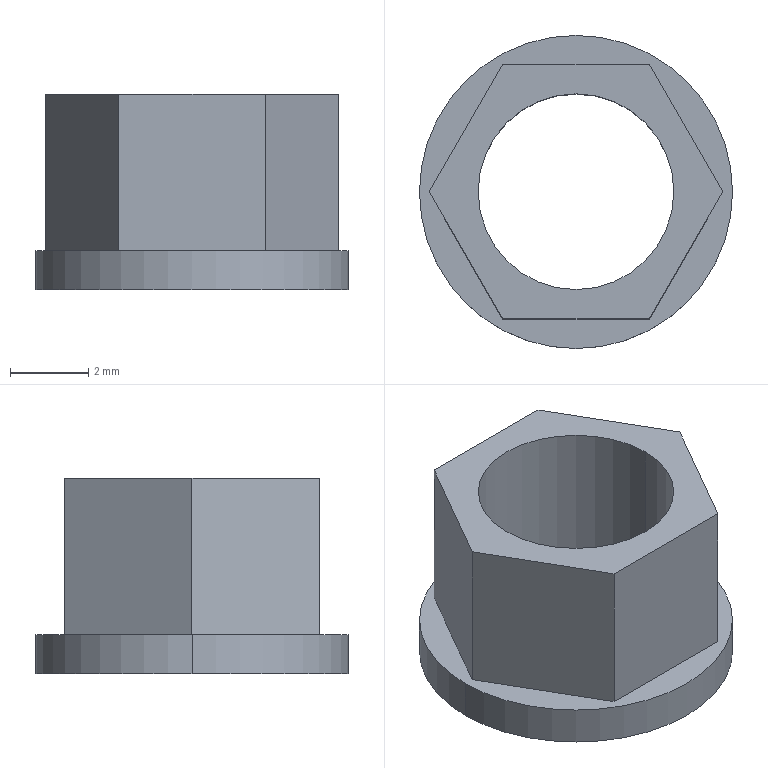Part | SolidWorks | features BaseBody 1 | 1 solid | 13 faces | box 8 x 8 x 5 mm | volume 98.449 mm3 | plane 9 | cylinder 4 | commonest cylinder face diameters 5 x2 8 x2
STEP:
#1=CARTESIAN_POINT('',(2.5,0.,0.));
#2=VERTEX_POINT('',#1);
#3=CARTESIAN_POINT('',(-2.5,0.,0.));
#4=VERTEX_POINT('',#3);
#5=CARTESIAN_POINT('',(0.,0.,0.));
#6=DIRECTION('',(0.,0.,1.));
#7=DIRECTION('',(-1.,0.,0.));
#8=AXIS2_PLACEMENT_3D('',#5,#6,#7);
#9=CIRCLE('',#8,2.5);
#10=EDGE_CURVE('',#2,#4,#9,.T.);
#11=ORIENTED_EDGE('',*,*,#10,.F.);
#12=CARTESIAN_POINT('',(2.5,0.,5.));
#13=VERTEX_POINT('',#12);
#14=CARTESIAN_POINT('',(2.5,0.,5.));
#15=DIRECTION('',(0.,0.,1.));
#16=VECTOR('',#15,1000.);
#17=LINE('',#14,#16);
#18=EDGE_CURVE('',#2,#13,#17,.T.);
#19=ORIENTED_EDGE('',*,*,#18,.T.);
#20=CARTESIAN_POINT('',(-2.5,0.,5.));
#21=VERTEX_POINT('',#20);
#22=CARTESIAN_POINT('',(0.,0.,5.));
#23=DIRECTION('',(0.,0.,-1.));
#24=DIRECTION('',(-1.,0.,0.));
#25=AXIS2_PLACEMENT_3D('',#22,#23,#24);
#26=CIRCLE('',#25,2.5);
#27=EDGE_CURVE('',#21,#13,#26,.T.);
#28=ORIENTED_EDGE('',*,*,#27,.F.);
#29=CARTESIAN_POINT('',(-2.5,0.,5.));
#30=DIRECTION('',(0.,0.,1.));
#31=VECTOR('',#30,1000.);
#32=LINE('',#29,#31);
#33=EDGE_CURVE('',#4,#21,#32,.T.);
#34=ORIENTED_EDGE('',*,*,#33,.F.);
#35=EDGE_LOOP('',(#11,#19,#28,#34));
#36=FACE_OUTER_BOUND('',#35,.T.);
#37=CARTESIAN_POINT('',(0.,0.,5.));
#38=DIRECTION('',(0.,0.,1.));
#39=DIRECTION('',(-1.,0.,0.));
#40=AXIS2_PLACEMENT_3D('',#37,#38,#39);
#41=CYLINDRICAL_SURFACE('',#40,2.5);
#42=ADVANCED_FACE('',(#36),#41,.F.);
#43=CARTESIAN_POINT('',(4.,0.,1.));
#44=VERTEX_POINT('',#43);
#45=CARTESIAN_POINT('',(-4.,0.,1.));
#46=VERTEX_POINT('',#45);
#47=CARTESIAN_POINT('',(0.,0.,1.));
#48=DIRECTION('',(0.,0.,1.));
#49=DIRECTION('',(-1.,0.,0.));
#50=AXIS2_PLACEMENT_3D('',#47,#48,#49);
#51=CIRCLE('',#50,4.);
#52=EDGE_CURVE('',#44,#46,#51,.T.);
#53=ORIENTED_EDGE('',*,*,#52,.F.);
#54=CARTESIAN_POINT('',(4.,0.,0.));
#55=VERTEX_POINT('',#54);
#56=CARTESIAN_POINT('',(4.,0.,0.));
#57=DIRECTION('',(0.,0.,-1.));
#58=VECTOR('',#57,1000.);
#59=LINE('',#56,#58);
#60=EDGE_CURVE('',#44,#55,#59,.T.);
#61=ORIENTED_EDGE('',*,*,#60,.T.);
#62=CARTESIAN_POINT('',(-4.,0.,0.));
#63=VERTEX_POINT('',#62);
#64=CARTESIAN_POINT('',(0.,0.,0.));
#65=DIRECTION('',(0.,0.,-1.));
#66=DIRECTION('',(-1.,0.,0.));
#67=AXIS2_PLACEMENT_3D('',#64,#65,#66);
#68=CIRCLE('',#67,4.);
#69=EDGE_CURVE('',#63,#55,#68,.T.);
#70=ORIENTED_EDGE('',*,*,#69,.F.);
#71=CARTESIAN_POINT('',(-4.,0.,0.));
#72=DIRECTION('',(0.,0.,-1.));
#73=VECTOR('',#72,1000.);
#74=LINE('',#71,#73);
#75=EDGE_CURVE('',#46,#63,#74,.T.);
#76=ORIENTED_EDGE('',*,*,#75,.F.);
#77=EDGE_LOOP('',(#53,#61,#70,#76));
#78=FACE_OUTER_BOUND('',#77,.T.);
#79=CARTESIAN_POINT('',(0.,0.,0.));
#80=DIRECTION('',(0.,0.,-1.));
#81=DIRECTION('',(-1.,0.,0.));
#82=AXIS2_PLACEMENT_3D('',#79,#80,#81);
#83=CYLINDRICAL_SURFACE('',#82,4.);
#84=ADVANCED_FACE('',(#78),#83,.T.);
#85=CARTESIAN_POINT('',(-1.876,-3.25,1.));
#86=VERTEX_POINT('',#85);
#87=CARTESIAN_POINT('',(-3.753,0.,1.));
#88=VERTEX_POINT('',#87);
#89=CARTESIAN_POINT('',(-3.284,-0.8125,1.));
#90=DIRECTION('',(-0.5,0.866,0.));
#91=VECTOR('',#90,1000.);
#92=LINE('',#89,#91);
#93=EDGE_CURVE('',#86,#88,#92,.T.);
#94=ORIENTED_EDGE('',*,*,#93,.F.);
#95=CARTESIAN_POINT('',(-1.876,-3.25,5.));
#96=VERTEX_POINT('',#95);
#97=CARTESIAN_POINT('',(-1.876,-3.25,1.));
#98=DIRECTION('',(0.,0.,1.));
#99=VECTOR('',#98,1000.);
#100=LINE('',#97,#99);
#101=EDGE_CURVE('',#86,#96,#100,.T.);
#102=ORIENTED_EDGE('',*,*,#101,.T.);
#103=CARTESIAN_POINT('',(-3.753,0.,5.));
#104=VERTEX_POINT('',#103);
#105=CARTESIAN_POINT('',(-1.876,-3.25,5.));
#106=DIRECTION('',(0.5,-0.866,0.));
#107=VECTOR('',#106,1000.);
#108=LINE('',#105,#107);
#109=EDGE_CURVE('',#104,#96,#108,.T.);
#110=ORIENTED_EDGE('',*,*,#109,.F.);
#111=CARTESIAN_POINT('',(-3.753,0.,1.));
#112=DIRECTION('',(0.,0.,1.));
#113=VECTOR('',#112,1000.);
#114=LINE('',#111,#113);
#115=EDGE_CURVE('',#88,#104,#114,.T.);
#116=ORIENTED_EDGE('',*,*,#115,.F.);
#117=EDGE_LOOP('',(#94,#102,#110,#116));
#118=FACE_OUTER_BOUND('',#117,.T.);
#119=CARTESIAN_POINT('',(-3.753,0.,1.));
#120=DIRECTION('',(-0.866,-0.5,0.));
#121=DIRECTION('',(-0.5,0.866,0.));
#122=AXIS2_PLACEMENT_3D('',#119,#120,#121);
#123=PLANE('',#122);
#124=ADVANCED_FACE('',(#118),#123,.T.);
#125=CARTESIAN_POINT('',(-1.876,3.25,1.));
#126=VERTEX_POINT('',#125);
#127=CARTESIAN_POINT('',(-2.345,2.438,1.));
#128=DIRECTION('',(0.5,0.866,0.));
#129=VECTOR('',#128,1000.);
#130=LINE('',#127,#129);
#131=EDGE_CURVE('',#88,#126,#130,.T.);
#132=ORIENTED_EDGE('',*,*,#131,.F.);
#133=ORIENTED_EDGE('',*,*,#115,.T.);
#134=CARTESIAN_POINT('',(-1.876,3.25,5.));
#135=VERTEX_POINT('',#134);
#136=CARTESIAN_POINT('',(-3.753,0.,5.));
#137=DIRECTION('',(-0.5,-0.866,0.));
#138=VECTOR('',#137,1000.);
#139=LINE('',#136,#138);
#140=EDGE_CURVE('',#135,#104,#139,.T.);
#141=ORIENTED_EDGE('',*,*,#140,.F.);
#142=CARTESIAN_POINT('',(-1.876,3.25,1.));
#143=DIRECTION('',(0.,0.,1.));
#144=VECTOR('',#143,1000.);
#145=LINE('',#142,#144);
#146=EDGE_CURVE('',#126,#135,#145,.T.);
#147=ORIENTED_EDGE('',*,*,#146,.F.);
#148=EDGE_LOOP('',(#132,#133,#141,#147));
#149=FACE_OUTER_BOUND('',#148,.T.);
#150=CARTESIAN_POINT('',(-1.876,3.25,1.));
#151=DIRECTION('',(-0.866,0.5,0.));
#152=DIRECTION('',(0.,0.,1.));
#153=AXIS2_PLACEMENT_3D('',#150,#151,#152);
#154=PLANE('',#153);
#155=ADVANCED_FACE('',(#149),#154,.T.);
#156=CARTESIAN_POINT('',(1.876,3.25,1.));
#157=VERTEX_POINT('',#156);
#158=CARTESIAN_POINT('',(0.9382,3.25,1.));
#159=DIRECTION('',(1.,0.,0.));
#160=VECTOR('',#159,1000.);
#161=LINE('',#158,#160);
#162=EDGE_CURVE('',#126,#157,#161,.T.);
#163=ORIENTED_EDGE('',*,*,#162,.F.);
#164=ORIENTED_EDGE('',*,*,#146,.T.);
#165=CARTESIAN_POINT('',(1.876,3.25,5.));
#166=VERTEX_POINT('',#165);
#167=CARTESIAN_POINT('',(-1.876,3.25,5.));
#168=DIRECTION('',(-1.,0.,0.));
#169=VECTOR('',#168,1000.);
#170=LINE('',#167,#169);
#171=EDGE_CURVE('',#166,#135,#170,.T.);
#172=ORIENTED_EDGE('',*,*,#171,.F.);
#173=CARTESIAN_POINT('',(1.876,3.25,1.));
#174=DIRECTION('',(0.,0.,1.));
#175=VECTOR('',#174,1000.);
#176=LINE('',#173,#175);
#177=EDGE_CURVE('',#157,#166,#176,.T.);
#178=ORIENTED_EDGE('',*,*,#177,.F.);
#179=EDGE_LOOP('',(#163,#164,#172,#178));
#180=FACE_OUTER_BOUND('',#179,.T.);
#181=CARTESIAN_POINT('',(1.876,3.25,1.));
#182=DIRECTION('',(0.,1.,0.));
#183=DIRECTION('',(1.,0.,0.));
#184=AXIS2_PLACEMENT_3D('',#181,#182,#183);
#185=PLANE('',#184);
#186=ADVANCED_FACE('',(#180),#185,.T.);
#187=CARTESIAN_POINT('',(3.753,0.,1.));
#188=VERTEX_POINT('',#187);
#189=CARTESIAN_POINT('',(3.284,0.8125,1.));
#190=DIRECTION('',(0.5,-0.866,0.));
#191=VECTOR('',#190,1000.);
#192=LINE('',#189,#191);
#193=EDGE_CURVE('',#157,#188,#192,.T.);
#194=ORIENTED_EDGE('',*,*,#193,.F.);
#195=ORIENTED_EDGE('',*,*,#177,.T.);
#196=CARTESIAN_POINT('',(3.753,0.,5.));
#197=VERTEX_POINT('',#196);
#198=CARTESIAN_POINT('',(1.876,3.25,5.));
#199=DIRECTION('',(-0.5,0.866,0.));
#200=VECTOR('',#199,1000.);
#201=LINE('',#198,#200);
#202=EDGE_CURVE('',#197,#166,#201,.T.);
#203=ORIENTED_EDGE('',*,*,#202,.F.);
#204=CARTESIAN_POINT('',(3.753,0.,1.));
#205=DIRECTION('',(0.,0.,1.));
#206=VECTOR('',#205,1000.);
#207=LINE('',#204,#206);
#208=EDGE_CURVE('',#188,#197,#207,.T.);
#209=ORIENTED_EDGE('',*,*,#208,.F.);
#210=EDGE_LOOP('',(#194,#195,#203,#209));
#211=FACE_OUTER_BOUND('',#210,.T.);
#212=CARTESIAN_POINT('',(3.753,0.,1.));
#213=DIRECTION('',(0.866,0.5,0.));
#214=DIRECTION('',(0.,0.,-1.));
#215=AXIS2_PLACEMENT_3D('',#212,#213,#214);
#216=PLANE('',#215);
#217=ADVANCED_FACE('',(#211),#216,.T.);
#218=CARTESIAN_POINT('',(1.876,-3.25,1.));
#219=VERTEX_POINT('',#218);
#220=CARTESIAN_POINT('',(2.345,-2.438,1.));
#221=DIRECTION('',(-0.5,-0.866,0.));
#222=VECTOR('',#221,1000.);
#223=LINE('',#220,#222);
#224=EDGE_CURVE('',#188,#219,#223,.T.);
#225=ORIENTED_EDGE('',*,*,#224,.F.);
#226=ORIENTED_EDGE('',*,*,#208,.T.);
#227=CARTESIAN_POINT('',(1.876,-3.25,5.));
#228=VERTEX_POINT('',#227);
#229=CARTESIAN_POINT('',(3.753,0.,5.));
#230=DIRECTION('',(0.5,0.866,0.));
#231=VECTOR('',#230,1000.);
#232=LINE('',#229,#231);
#233=EDGE_CURVE('',#228,#197,#232,.T.);
#234=ORIENTED_EDGE('',*,*,#233,.F.);
#235=CARTESIAN_POINT('',(1.876,-3.25,1.));
#236=DIRECTION('',(0.,0.,1.));
#237=VECTOR('',#236,1000.);
#238=LINE('',#235,#237);
#239=EDGE_CURVE('',#219,#228,#238,.T.);
#240=ORIENTED_EDGE('',*,*,#239,.F.);
#241=EDGE_LOOP('',(#225,#226,#234,#240));
#242=FACE_OUTER_BOUND('',#241,.T.);
#243=CARTESIAN_POINT('',(1.876,-3.25,1.));
#244=DIRECTION('',(0.866,-0.5,0.));
#245=DIRECTION('',(0.,0.,-1.));
#246=AXIS2_PLACEMENT_3D('',#243,#244,#245);
#247=PLANE('',#246);
#248=ADVANCED_FACE('',(#242),#247,.T.);
#249=CARTESIAN_POINT('',(-0.9382,-3.25,1.));
#250=DIRECTION('',(-1.,0.,0.));
#251=VECTOR('',#250,1000.);
#252=LINE('',#249,#251);
#253=EDGE_CURVE('',#219,#86,#252,.T.);
#254=ORIENTED_EDGE('',*,*,#253,.F.);
#255=ORIENTED_EDGE('',*,*,#239,.T.);
#256=CARTESIAN_POINT('',(1.876,-3.25,5.));
#257=DIRECTION('',(1.,0.,0.));
#258=VECTOR('',#257,1000.);
#259=LINE('',#256,#258);
#260=EDGE_CURVE('',#96,#228,#259,.T.);
#261=ORIENTED_EDGE('',*,*,#260,.F.);
#262=ORIENTED_EDGE('',*,*,#101,.F.);
#263=EDGE_LOOP('',(#254,#255,#261,#262));
#264=FACE_OUTER_BOUND('',#263,.T.);
#265=CARTESIAN_POINT('',(-1.876,-3.25,1.));
#266=DIRECTION('',(0.,-1.,0.));
#267=DIRECTION('',(-1.,0.,0.));
#268=AXIS2_PLACEMENT_3D('',#265,#266,#267);
#269=PLANE('',#268);
#270=ADVANCED_FACE('',(#264),#269,.T.);
#271=ORIENTED_EDGE('',*,*,#27,.T.);
#272=CARTESIAN_POINT('',(0.,0.,5.));
#273=DIRECTION('',(0.,0.,-1.));
#274=DIRECTION('',(-1.,0.,0.));
#275=AXIS2_PLACEMENT_3D('',#272,#273,#274);
#276=CIRCLE('',#275,2.5);
#277=EDGE_CURVE('',#13,#21,#276,.T.);
#278=ORIENTED_EDGE('',*,*,#277,.T.);
#279=EDGE_LOOP('',(#271,#278));
#280=FACE_BOUND('',#279,.T.);
#281=ORIENTED_EDGE('',*,*,#260,.T.);
#282=ORIENTED_EDGE('',*,*,#233,.T.);
#283=ORIENTED_EDGE('',*,*,#202,.T.);
#284=ORIENTED_EDGE('',*,*,#171,.T.);
#285=ORIENTED_EDGE('',*,*,#140,.T.);
#286=ORIENTED_EDGE('',*,*,#109,.T.);
#287=EDGE_LOOP('',(#281,#282,#283,#284,#285,#286));
#288=FACE_OUTER_BOUND('',#287,.T.);
#289=CARTESIAN_POINT('',(0.,0.,5.));
#290=DIRECTION('',(0.,0.,1.));
#291=DIRECTION('',(1.,0.,0.));
#292=AXIS2_PLACEMENT_3D('',#289,#290,#291);
#293=PLANE('',#292);
#294=ADVANCED_FACE('',(#280,#288),#293,.T.);
#295=CARTESIAN_POINT('',(0.,0.,0.));
#296=DIRECTION('',(0.,0.,1.));
#297=DIRECTION('',(-1.,0.,0.));
#298=AXIS2_PLACEMENT_3D('',#295,#296,#297);
#299=CIRCLE('',#298,2.5);
#300=EDGE_CURVE('',#4,#2,#299,.T.);
#301=ORIENTED_EDGE('',*,*,#300,.T.);
#302=ORIENTED_EDGE('',*,*,#10,.T.);
#303=EDGE_LOOP('',(#301,#302));
#304=FACE_BOUND('',#303,.T.);
#305=ORIENTED_EDGE('',*,*,#69,.T.);
#306=CARTESIAN_POINT('',(0.,0.,0.));
#307=DIRECTION('',(0.,0.,-1.));
#308=DIRECTION('',(-1.,0.,0.));
#309=AXIS2_PLACEMENT_3D('',#306,#307,#308);
#310=CIRCLE('',#309,4.);
#311=EDGE_CURVE('',#55,#63,#310,.T.);
#312=ORIENTED_EDGE('',*,*,#311,.T.);
#313=EDGE_LOOP('',(#305,#312));
#314=FACE_OUTER_BOUND('',#313,.T.);
#315=CARTESIAN_POINT('',(0.,0.,0.));
#316=DIRECTION('',(0.,0.,1.));
#317=DIRECTION('',(1.,0.,0.));
#318=AXIS2_PLACEMENT_3D('',#315,#316,#317);
#319=PLANE('',#318);
#320=ADVANCED_FACE('',(#304,#314),#319,.F.);
#321=ORIENTED_EDGE('',*,*,#93,.T.);
#322=ORIENTED_EDGE('',*,*,#131,.T.);
#323=ORIENTED_EDGE('',*,*,#162,.T.);
#324=ORIENTED_EDGE('',*,*,#193,.T.);
#325=ORIENTED_EDGE('',*,*,#224,.T.);
#326=ORIENTED_EDGE('',*,*,#253,.T.);
#327=EDGE_LOOP('',(#321,#322,#323,#324,#325,#326));
#328=FACE_BOUND('',#327,.T.);
#329=CARTESIAN_POINT('',(0.,0.,1.));
#330=DIRECTION('',(0.,0.,1.));
#331=DIRECTION('',(-1.,0.,0.));
#332=AXIS2_PLACEMENT_3D('',#329,#330,#331);
#333=CIRCLE('',#332,4.);
#334=EDGE_CURVE('',#46,#44,#333,.T.);
#335=ORIENTED_EDGE('',*,*,#334,.T.);
#336=ORIENTED_EDGE('',*,*,#52,.T.);
#337=EDGE_LOOP('',(#335,#336));
#338=FACE_OUTER_BOUND('',#337,.T.);
#339=CARTESIAN_POINT('',(0.,0.,1.));
#340=DIRECTION('',(0.,0.,1.));
#341=DIRECTION('',(1.,0.,0.));
#342=AXIS2_PLACEMENT_3D('',#339,#340,#341);
#343=PLANE('',#342);
#344=ADVANCED_FACE('',(#328,#338),#343,.T.);
#345=ORIENTED_EDGE('',*,*,#60,.F.);
#346=ORIENTED_EDGE('',*,*,#334,.F.);
#347=ORIENTED_EDGE('',*,*,#75,.T.);
#348=ORIENTED_EDGE('',*,*,#311,.F.);
#349=EDGE_LOOP('',(#345,#346,#347,#348));
#350=FACE_OUTER_BOUND('',#349,.T.);
#351=CARTESIAN_POINT('',(0.,0.,0.));
#352=DIRECTION('',(0.,0.,-1.));
#353=DIRECTION('',(-1.,0.,0.));
#354=AXIS2_PLACEMENT_3D('',#351,#352,#353);
#355=CYLINDRICAL_SURFACE('',#354,4.);
#356=ADVANCED_FACE('',(#350),#355,.T.);
#357=ORIENTED_EDGE('',*,*,#18,.F.);
#358=ORIENTED_EDGE('',*,*,#300,.F.);
#359=ORIENTED_EDGE('',*,*,#33,.T.);
#360=ORIENTED_EDGE('',*,*,#277,.F.);
#361=EDGE_LOOP('',(#357,#358,#359,#360));
#362=FACE_OUTER_BOUND('',#361,.T.);
#363=CARTESIAN_POINT('',(0.,0.,5.));
#364=DIRECTION('',(0.,0.,1.));
#365=DIRECTION('',(-1.,0.,0.));
#366=AXIS2_PLACEMENT_3D('',#363,#364,#365);
#367=CYLINDRICAL_SURFACE('',#366,2.5);
#368=ADVANCED_FACE('',(#362),#367,.F.);
#369=CLOSED_SHELL('',(#42,#84,#124,#155,#186,#217,#248,#270,#294,#320,#344,#356,#368));
#370=MANIFOLD_SOLID_BREP('',#369);
#371=CARTESIAN_POINT('',(0.,0.,0.));
#372=DIRECTION('',(0.,0.,1.));
#373=DIRECTION('',(1.,0.,0.));
#374=AXIS2_PLACEMENT_3D('',#371,#372,#373);
#375=(LENGTH_UNIT()NAMED_UNIT(*)SI_UNIT(.MILLI.,.METRE.));
#376=UNCERTAINTY_MEASURE_WITH_UNIT(LENGTH_MEASURE(0.00001),#375,'','');
#377=(NAMED_UNIT(*)PLANE_ANGLE_UNIT()SI_UNIT($,.RADIAN.));
#378=(NAMED_UNIT(*)SI_UNIT($,.STERADIAN.)SOLID_ANGLE_UNIT());
#379=(GEOMETRIC_REPRESENTATION_CONTEXT(3)GLOBAL_UNCERTAINTY_ASSIGNED_CONTEXT((#376))GLOBAL_UNIT_ASSIGNED_CONTEXT((#375,#377,#378))REPRESENTATION_CONTEXT('',''));
#380=ADVANCED_BREP_SHAPE_REPRESENTATION('',(#370,#374),#379);